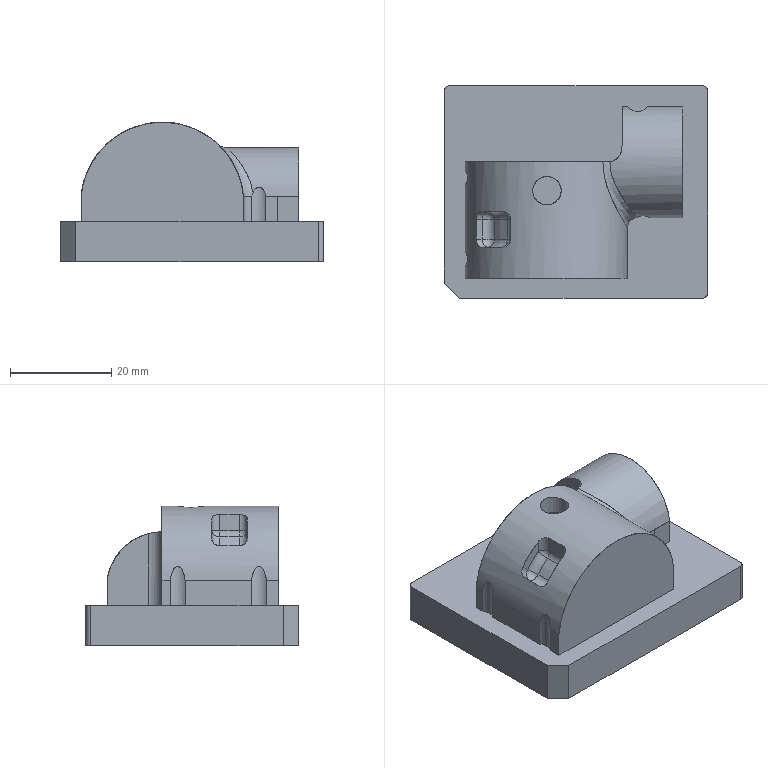NC program | PowerMill | posted with a generic post | part box 52 x 42 x 27.622 mm
Lines 1 to 940 of 322299:
%
O0001
N104 ( POWERMILL CB  : 2026004.0)
N105 ( POST VER      : 2026.0.0.5161)
N106 ( OPTION FILE   : FANUC)
N107 ( OUTPUT WORKPLANE : WORLD)
N108 (  )
N109 ( TOOL LIST )
N110 (---------------------------------------)
N111 ( NO. | ID        | DIA.| TIP RAD|LENGTH)
N112 (---------------------------------------)
N113 (    1|D10C_1_1_1 |10.0 |  0.0   |83.08 )
N114 (    2|D4C_1_1    | 4.0 |  0.0   | 74.8 )
N115 (   28|D2C_1_1    | 2.0 |  0.0   |67.72 )
N116 (    3|D10_1_1_1  |10.0 |  0.0   | 82.8 )
N117 (    7|R2_1_1     | 4.0 |  2.0   |71.76 )
N118 (   10|D3_1_1     | 3.0 |  0.0   |74.88 )
N119 (    4|R1_1_1     | 2.0 |  1.0   |64.72 )
N120 (   13|TEXT_D4_1_1| 4.0 |  0.3   |74.88 )
N121 (---------------------------------------)
N122 (  )
N123 ( NUMBER OF TOOLPATHS: 13.0 )
N124 ( ESTIMATED PROGRAM DURATION: 0 HOURS 30 MIN 34 SEC)
N125 (  )
N126 G00 G21 G80 G40 G17
N127 G90
N128 G54
N129 G53 Z0.0
N130 (---------------)
N131 ( START TOOLPATH : 精公开粗01-扫面平行-D10C )
N132 (---------------)
N133 ( TOOL NO.    :1 )
N134 ( TOOL TYPE   : ENDMILL)
N135 ( TOOL ID     : D10C_1_1_1)
N136 ( TOOL DIA    : 10.0 LENGTH 83.08)
N137 T1
N138 M6
N139 S8000 M03
N140 G00 G90 X0.0 Y0.0
N141 G43 Z10.2 H1
N142
N143 G05 P10000 R4
N144 X28.78 Y23.78
N145 Z1.132
N146 G01 Z-0.068 F6000.0
N147 X-28.78 F10000.0
N148 Y17.835
N149 X28.78
N150 Y11.89
N151 X-28.78
N152 Y5.945
N153 X28.78
N154 Y0.0
N155 X-28.78
N156 Y-5.945
N157 X28.78
N158 Y-11.89
N159 X-28.78
N160 Y-17.835
N161 X28.78
N162 Y-23.78
N163 X-28.78
N164 X-33.78
N165 G00 Z10.2
N166 G05 P0
N167 (---------------)
N168 ( END TOOLPATH : 精公开粗01-扫面平行-D10C )
N169 (---------------)
N170 ( START TOOLPATH : 精公开粗01-外形偏置-D10C )
N171 (---------------)
N172 G00 X-0.4155 Y-0.186 Z9.882
N173 G05 P10000 R4
N174 X2.3999 Y-30.215
N175 Z0.6838
N176 G01 Z-0.5162 F6000.0
N177 Y-29.6875 F10000.0
N178 G03 X-2.3476 Y-24.94 I-4.7475 J0.0
N179 G01 X-28.709
N180 G02 X-29.709 Y-23.94 I0.0 J1.0
N181 G01 Y23.568
N182 G02 X-28.709 Y24.568 I1.0 J0.0
N183 G01 X27.878
N184 G02 X28.878 Y23.568 I0.0 J-1.0
N185 G01 Y-0.2313
N186 X22.9872 Y-0.2546
N187 X17.4174 Y-0.2767
N188 X17.3721 Y11.1517
N189 G03 X15.2157 Y13.0657 I-1.9344 J-0.0077
N190 G03 X13.5525 Y10.7105 I0.222 J-1.9217
N191 G01 X14.089 Y8.3779
N192 G02 X14.5687 Y3.9884 I-18.4003 J-4.2319
N193 G01 X14.4374 Y-11.7373
N194 G03 X15.5858 Y-12.9585 I1.2128 J-0.0101
N195 G01 X16.1164 Y-12.9867
N196 G03 X17.4626 Y-11.705 I0.0678 J1.2766
N197 G01 X17.4174 Y-0.2767
N198 X22.9872 Y-0.2546
N199 Y-17.0492
N200 G02 X21.0004 Y-19.0491 I-2.0 J0.0
N201 G01 X10.7449 Y-19.1171
N202 G02 X8.7319 Y-17.0871 I-0.0133 J2.0
N203 G01 X9.0472 Y3.9049
N204 G03 X-5.0505 Y17.6259 I-13.5283 J0.2032
N205 G01 X-7.8978 Y17.506
N206 G03 X-21.0318 Y3.2025 I0.5776 J-13.7122
N207 G01 X-20.1558 Y-17.1107
N208 G02 X-21.6983 Y-18.9728 I-1.8015 J-0.0776
N209 G01 X-22.0663 Y-19.0263
N210 G02 X-24.1285 Y-17.2253 I-0.259 J1.7846
N211 G01 X-23.8181 Y16.6955
N212 G02 X-21.8182 Y18.6772 I1.9999 J-0.0183
N213 G01 X20.9872
N214 G02 X22.9872 Y16.6772 I0.0 J-2.0
N215 G01 Y-0.2546
N216 X28.878 Y-0.2313
N217 Y-23.94
N218 G02 X27.878 Y-24.94 I-1.0 J0.0
N219 G01 X-2.3476
N220 X-2.3491 Y-22.432
N221 X-9.3099 Y-22.4361
N222 X-10.0833 Y-22.3648
N223 X-10.8568 Y-22.1889
N224 X-11.6302 Y-21.889
N225 X-12.4036 Y-21.4357
N226 X-12.8677 Y-21.0685
N227 X-13.177 Y-20.7678
N228 X-13.5777 Y-20.2951
N229 X-14.06 Y-19.5217
N230 X-14.3759 Y-18.7482
N231 X-14.5593 Y-17.9748
N232 X-14.6224 Y-17.2014
N233 X-14.6405 Y-13.3343
N234 X-14.6103 Y-12.5608
N235 X-14.6019 Y-10.2405
N236 X-14.6459 Y-9.4671
N237 X-14.6072 Y-0.9594
N238 X-14.6415 Y1.3609
N239 X-14.6073 Y5.228
N240 X-14.6321 Y6.0014
N241 X-14.5643 Y6.7748
N242 X-14.3779 Y7.5483
N243 X-14.0567 Y8.3217
N244 X-13.576 Y9.0951
N245 X-13.177 Y9.5623
N246 X-12.8477 Y9.8685
N247 X-12.4036 Y10.223
N248 X-11.6892 Y10.642
N249 X-10.8568 Y10.9701
N250 X-10.0833 Y11.1451
N251 X-9.3099 Y11.2163
N252 X-2.3491 Y11.2116
N253 X-1.5756 Y11.1233
N254 X-0.8022 Y10.9323
N255 X-0.0807 Y10.642
N256 X0.7446 Y10.1386
N257 X1.0811 Y9.8685
N258 X1.5181 Y9.4317
N259 X1.7998 Y9.0951
N260 X2.2915 Y8.3058
N261 X2.6078 Y7.5483
N262 X2.7924 Y6.7748
N263 X2.8611 Y6.0014
N264 X2.8419 Y5.228
N265 X2.8774 Y0.5874
N266 X2.8333 Y-0.9594
N267 Y-0.9666
N268 Y-11.7874
N269 X2.8744 Y-13.3343
N270 X2.8668 Y-17.2014
N271 X2.8067 Y-17.9748
N272 X2.6234 Y-18.7482
N273 X2.303 Y-19.5217
N274 X1.826 Y-20.2951
N275 X1.5181 Y-20.6639
N276 X1.1107 Y-21.0685
N277 X0.7446 Y-21.3656
N278 X-0.0286 Y-21.8419
N279 X-0.8022 Y-22.1586
N280 X-1.5756 Y-22.348
N281 X-2.3491 Y-22.432
N282 X-2.3476 Y-24.94
N283 G00 Z3.2856
N284 G01 X2.3999 Y-30.215
N285 G00 Z0.2856
N286 G01 Z-0.9144 F6000.0
N287 Y-29.6875 F10000.0
N288 G03 X-2.3476 Y-24.94 I-4.7475 J0.0
N289 G01 X-28.709
N290 G02 X-29.709 Y-23.94 I0.0 J1.0
N291 G01 Y23.568
N292 G02 X-28.709 Y24.568 I1.0 J0.0
N293 G01 X27.878
N294 G02 X28.878 Y23.568 I0.0 J-1.0
N295 G01 Y-0.2845
N296 X22.9872 Y-0.2788
N297 X17.0576 Y-0.273
N298 X17.0697 Y12.19
N299 G03 X16.5006 Y12.7597 I-0.5692 J0.0005
N300 G01 X15.1565 Y12.7598
N301 G03 X14.8346 Y12.2613 I-0.0001 J-0.3531
N302 G01 X15.0028 Y11.889
N303 G02 X16.6841 Y3.5678 I-17.346 J-7.8354
N304 G01 X16.2681 Y-12.7268
N305 G03 X16.5196 Y-13.0878 I0.3713 J-0.0095
N306 G01 X16.5426 Y-13.0956
N307 G03 X17.0455 Y-12.736 I0.1226 J0.3599
N308 G01 X17.0576 Y-0.273
N309 X22.9872 Y-0.2788
N310 Y-17.0492
N311 G02 X21.0033 Y-19.0491 I-2.0 J0.0
N312 G01 X12.2098 Y-19.1201
N313 G02 X10.1945 Y-17.0647 I-0.0161 J1.9999
N314 G01 X10.7699 Y3.6831
N315 G03 X-1.6795 Y17.1746 I-13.1402 J0.3644
N316 G01 X-8.0692 Y17.5108
N317 G03 X-22.4796 Y3.2616 I-0.7199 J-13.6832
N318 G01 X-21.6108 Y-17.7521
N319 G02 X-22.5168 Y-18.7408 I-0.9496 J-0.0393
N320 G01 X-23.1117 Y-18.7681
N321 G02 X-24.1057 Y-17.8108 I-0.0436 J0.9494
N322 G01 X-23.8181 Y16.6938
N323 G02 X-21.8182 Y18.6772 I1.9999 J-0.0166
N324 G01 X20.9872
N325 G02 X22.9872 Y16.6772 I0.0 J-2.0
N326 G01 Y-0.2788
N327 X28.878 Y-0.2845
N328 Y-23.94
N329 G02 X27.878 Y-24.94 I-1.0 J0.0
N330 G01 X-0.7722
N331 X-0.8022 Y-22.432
N332 X-1.5756 Y-22.4412
N333 X-10.0833
N334 X-10.8568 Y-22.4363
N335 X-11.6302 Y-22.3544
N336 X-12.4036 Y-22.1649
N337 X-13.1939 Y-21.8419
N338 X-13.9505 Y-21.3731
N339 X-14.3262 Y-21.0685
N340 X-14.7239 Y-20.6762
N341 X-15.0415 Y-20.2951
N342 X-15.4973 Y-19.5621
N343 X-15.8358 Y-18.7482
N344 X-16.0184 Y-17.9748
N345 X-16.0829 Y-17.2014
N346 X-16.0644 Y-14.1077
N347 X-16.0897 Y-13.3343
N348 X-16.0907 Y6.0014
N349 X-16.0284 Y6.7748
N350 X-15.8421 Y7.5483
N351 X-15.5215 Y8.3217
N352 X-15.0371 Y9.0951
N353 X-14.7239 Y9.4705
N354 X-14.3198 Y9.8685
N355 X-13.9505 Y10.1626
N356 X-13.177 Y10.6358
N357 X-12.4036 Y10.9477
N358 X-11.6302 Y11.1341
N359 X-10.8568 Y11.2158
N360 X-10.0833 Y11.2213
N361 X-1.5756
N362 X-0.8022 Y11.2116
N363 X-0.0288 Y11.1164
N364 X0.7446 Y10.9135
N365 X1.3993 Y10.642
N366 X2.2915 Y10.083
N367 X2.5549 Y9.8685
N368 X3.0649 Y9.3467
N369 X3.27 Y9.0951
N370 X3.7539 Y8.3217
N371 X4.0784 Y7.5483
N372 X4.2652 Y6.7748
N373 X4.3314 Y6.0014
N374 X4.3208 Y5.228
N375 X4.3392 Y2.9077
N376 X4.3034 Y-1.7329
N377 X4.306 Y-12.5608
N378 X4.3287 Y-13.3343
N379 X4.3095 Y-14.1077
N380 Y-14.1154
N381 X4.3286 Y-17.2014
N382 X4.2638 Y-17.9748
N383 X4.0806 Y-18.7482
N384 X3.7637 Y-19.5217
N385 X3.2835 Y-20.2951
N386 X3.0649 Y-20.5654
N387 X2.5735 Y-21.0685
N388 X2.2915 Y-21.3024
N389 X1.4359 Y-21.8419
N390 X0.7446 Y-22.1331
N391 X-0.0288 Y-22.3371
N392 X-0.8022 Y-22.432
N393 X-0.7722 Y-24.94
N394 X-2.3476
N395 G00 Z2.8874
N396 G01 X2.3999 Y-30.215
N397 G00 Z-0.1126
N398 G01 Z-1.3126 F6000.0
N399 Y-29.6875 F10000.0
N400 G03 X-2.3476 Y-24.94 I-4.7475 J0.0
N401 G01 X-28.709
N402 G02 X-29.709 Y-23.94 I0.0 J1.0
N403 G01 Y23.568
N404 G02 X-28.709 Y24.568 I1.0 J0.0
N405 G01 X27.878
N406 G02 X28.878 Y23.568 I0.0 J-1.0
N407 G01 Y-0.518
N408 X23.0842 Y-0.5088
N409 X17.7571 Y-0.5003
N410 X17.7771 Y12.1344
N411 G03 X16.4479 Y13.4671 I-1.3306 J0.0021
N412 G01 X16.1198 Y13.4675
N413 G03 X15.3545 Y12.3375 I-0.0009 J-0.8236
N414 G01 X15.6519 Y11.5956
N415 G02 X16.8882 Y4.9198 I-16.0082 J-6.4169
N416 G01 X16.6172 Y-13.1236
N417 G03 X17.0637 Y-13.5815 I0.4511 J-0.0068
N418 G01 X17.283 Y-13.5838
N419 G03 X17.737 Y-13.135 I0.0045 J0.4495
N420 G01 X17.7571 Y-0.5003
N421 X23.0842 Y-0.5088
N422 Y-17.7235
N423 G02 X21.6615 Y-19.1462 I-1.4227 J0.0
N424 G01 X12.4578 Y-19.1463
N425 G02 X11.1881 Y-17.7948 I0.0 J1.2722
N426 G01 X11.1976 Y-17.6086
N427 X11.5863 Y4.9572
N428 G03 X-0.2272 Y17.169 I-12.0047 J0.2068
N429 G01 X-10.8025 Y17.3375
N430 G03 X-23.3444 Y4.7809 I-0.1966 J-12.3455
N431 G01 X-22.9698 Y-17.1238
N432 X-22.8718 Y-18.4412
N433 G02 X-23.2256 Y-18.837 I-0.3667 J-0.0283
N434 G01 X-23.5239 Y-18.8474
N435 G02 X-23.9045 Y-18.48 I-0.0128 J0.3675
N436 G01 X-23.9152 Y17.3511
N437 G02 X-22.4925 Y18.7742 I1.4227 J0.0004
N438 G01 X21.6615
N439 G02 X23.0842 Y17.3515 I0.0 J-1.4227
N440 G01 Y-0.5088
N441 X28.878 Y-0.518
N442 Y-23.94
N443 G02 X27.878 Y-24.94 I-1.0 J0.0
N444 G01 X0.418
N445 X0.2612 Y-22.4231
N446 X-0.0288 Y-22.4412
N447 X-11.6302
N448 X-12.4036 Y-22.4056
N449 X-13.177 Y-22.2655
N450 X-13.9505 Y-22.003
N451 X-14.297 Y-21.8419
N452 X-14.7239 Y-21.601
N453 X-15.4287 Y-21.0685
N454 X-16.137 Y-20.2951
N455 X-16.2707 Y-20.1076
N456 X-16.6157 Y-19.5217
N457 X-16.934 Y-18.7482
N458 X-17.1168 Y-17.9748
N459 X-17.1785 Y-17.2014
N460 X-17.1744 Y-14.1077
N461 X-17.1585 Y-12.5608
N462 X-17.1779 Y-9.4671
N463 X-17.1614 Y-0.186
N464 X-17.1782 Y0.5874
N465 X-17.1707 Y6.0014
N466 X-17.1024 Y6.7748
N467 X-16.9162 Y7.5483
N468 X-16.5963 Y8.3217
N469 X-16.2707 Y8.8703
N470 X-16.1117 Y9.0951
N471 X-15.4973 Y9.7733
N472 X-14.7239 Y10.3707
N473 X-14.2483 Y10.642
N474 X-13.9505 Y10.7779
N475 X-13.177 Y11.0406
N476 X-12.4036 Y11.1831
N477 X-11.6302 Y11.2213
N478 X-0.0288 Y11.2214
N479 X0.7446 Y11.1717
N480 X1.5181 Y11.0156
N481 X2.4979 Y10.642
N482 X3.0649 Y10.3117
N483 X3.6435 Y9.8685
N484 X3.8383 Y9.686
N485 X4.3612 Y9.0951
N486 X4.6118 Y8.7226
N487 X4.8439 Y8.3217
N488 X5.1639 Y7.5483
N489 X5.3525 Y6.7748
N490 X5.4166 Y6.0014
N491 X5.4212 Y2.9077
N492 X5.3948 Y-0.9594
N493 Y-12.5608
N494 X5.3952 Y-12.5702
N495 X5.4238 Y-13.3343
N496 X5.4247 Y-17.2014
N497 X5.3624 Y-17.9748
N498 X5.1795 Y-18.7482
N499 X4.8619 Y-19.5217
N500 X4.6118 Y-19.9596
N501 X4.3822 Y-20.2951
N502 X3.8383 Y-20.9144
N503 X3.6741 Y-21.0685
N504 X3.0649 Y-21.5384
N505 X2.5426 Y-21.8419
N506 X2.2915 Y-21.9626
N507 X1.5181 Y-22.2387
N508 X0.7446 Y-22.393
N509 X0.2612 Y-22.4231
N510 X0.418 Y-24.94
N511 X-2.3476
N512 G00 Z2.4892
N513 G01 X2.3999 Y-30.215
N514 G00 Z-0.5108
N515 G01 Z-1.7108 F6000.0
N516 Y-29.6875 F10000.0
N517 G03 X-2.3476 Y-24.94 I-4.7475 J0.0
N518 G01 X-28.709
N519 G02 X-29.709 Y-23.94 I0.0 J1.0
N520 G01 Y23.568
N521 G02 X-28.709 Y24.568 I1.0 J0.0
N522 G01 X27.878
N523 G02 X28.878 Y23.568 I0.0 J-1.0
N524 G01 Y-0.1777
N525 X23.1783 Y-0.1895
N526 X18.5438 Y-0.199
N527 X18.5172 Y12.6516
N528 G03 X16.6909 Y14.2143 I-1.5844 J-0.0032
N529 G03 X15.4212 Y12.1734 I0.2419 J-1.5659
N530 G01 X15.9354 Y10.5368
N531 G02 X16.6565 Y5.8812 I-14.9633 J-4.7014
N532 G01 X16.7119 Y-13.0537
N533 G03 X17.5048 Y-13.8443 I0.7929 J0.0023
N534 G01 X17.7773
N535 G03 X18.5703 Y-13.0497 I0.0 J0.7929
N536 G01 X18.5438 Y-0.199
N537 X23.1783 Y-0.1895
N538 Y-18.8932
N539 G02 X22.8312 Y-19.2403 I-0.3471 J0.0
N540 G01 X12.1493 Y-19.2404
N541 G02 X11.8751 Y-18.9269 I0.0 J0.2767
N542 G01 X11.929 Y-18.5253
N543 G03 X12.112 Y-15.7107 I-20.433 J2.7418
N544 G01 X12.1006 Y-12.4824
N545 X12.0566 Y5.8315
N546 G03 X0.7861 Y17.0039 I-11.1995 J-0.0269
N547 G01 X-12.3889 Y16.9203
N548 X-13.0327 Y16.9096
N549 X-13.5164 Y16.8882
N550 X-13.9983 Y16.8402
N551 X-14.1741 Y16.8179
N552 G03 X-16.2787 Y16.3267 I1.3322 J-10.4639
N553 G01 X-16.4753 Y16.259
N554 X-16.9889 Y16.0651
N555 X-17.4903 Y15.8416
N556 X-17.6232 Y15.7777
N557 X-17.9323 Y15.6215
N558 X-18.2352 Y15.4536
N559 X-18.314 Y15.4079
N560 G03 X-21.1188 Y13.0623 I5.3868 J-9.2909
N561 G01 X-21.2302 Y12.9309
N562 G03 X-22.4592 Y11.1191 I7.802 J-6.615
N563 G01 X-22.495 Y11.0517
N564 X-22.7031 Y10.6365
N565 X-22.8908 Y10.2117
N566 X-22.9648 Y10.0326
N567 G03 X-23.4415 Y8.5639 I9.1626 J-3.7856
N568 G01 X-23.4708 Y8.4419
N569 G03 X-23.7434 Y6.5319 I9.9814 J-2.3991
N570 G01 X-23.7604 Y6.1656
N571 X-23.7859 Y-7.0983
N572 X-23.7679 Y-17.3085
N573 X-23.7652 Y-17.4079
N574 X-23.6871 Y-18.4372
N575 X-23.6293 Y-19.0061
N576 X-23.6475 Y-19.0997
N577 X-23.7148 Y-19.1672
N578 X-23.7447 Y-19.1832
N579 G02 X-24.0076 Y-19.0257 I-0.0842 J0.1575
N580 G01 X-24.0093 Y18.5212
N581 G02 X-23.6622 Y18.8683 I0.3471 J0.0
N582 G01 X22.8312
N583 G02 X23.1783 Y18.5212 I0.0 J-0.3471
N584 G01 Y-0.1895
N585 X28.878 Y-0.1777
N586 Y-23.94
N587 G02 X27.878 Y-24.94 I-1.0 J0.0
N588 G01 X0.945
N589 X0.8413 Y-22.4372
N590 X0.7446 Y-22.4412
N591 X-12.4036
N592 X-13.177 Y-22.4173
N593 X-13.9505 Y-22.2955
N594 X-14.7239 Y-22.0533
N595 X-15.1937 Y-21.8419
N596 X-15.4973 Y-21.6728
N597 X-16.2707 Y-21.1106
N598 X-17.0293 Y-20.2951
N599 X-17.5083 Y-19.5217
N600 X-17.8243 Y-18.7482
N601 X-18.0071 Y-17.9748
N602 X-18.0705 Y-17.2014
N603 X-18.0513 Y-11.014
N604 X-18.0793 Y-9.4671
N605 X-18.0796 Y-4.8266
N606 X-18.0566 Y-2.5063
N607 X-18.064 Y6.0014
N608 X-17.9972 Y6.7748
N609 X-17.8113 Y7.5483
N610 X-17.4918 Y8.3217
N611 X-17.0442 Y9.0447
N612 X-16.2941 Y9.8685
N613 X-15.4973 Y10.4502
N614 X-15.1511 Y10.642
N615 X-14.7239 Y10.8331
N616 X-13.9505 Y11.0751
N617 X-13.177 Y11.1983
N618 X-12.4036 Y11.2214
N619 X0.7446
N620 X1.5181 Y11.1904
N621 X2.2915 Y11.0547
N622 X3.0649 Y10.797
N623 X3.4073 Y10.642
N624 X3.8383 Y10.3985
N625 X4.5503 Y9.8685
N626 X5.2645 Y9.0951
N627 X5.7482 Y8.3217
N628 X6.0676 Y7.5483
N629 X6.2533 Y6.7748
N630 X6.3197 Y6.0014
N631 X6.2994 Y5.228
N632 X6.317 Y0.5874
N633 X6.2997 Y-0.9594
N634 X6.2994 Y-12.5608
N635 X6.2995 Y-12.5667
N636 X6.3174 Y-13.3343
N637 X6.315 Y-17.2014
N638 X6.2515 Y-17.9748
N639 X6.0687 Y-18.7482
N640 X5.7527 Y-19.5217
N641 X5.2738 Y-20.2951
N642 X4.6118 Y-21.0251
N643 X3.8383 Y-21.6139
N644 X3.4382 Y-21.8419
N645 X3.0649 Y-22.0143
N646 X2.2915 Y-22.2706
N647 X1.5181 Y-22.4092
N648 X0.8413 Y-22.4372
N649 X0.945 Y-24.94
N650 X-2.3476
N651 G00 Z2.091
N652 G01 X2.3999 Y-30.215
N653 G00 Z-0.909
N654 G01 Z-2.109 F6000.0
N655 Y-29.6875 F10000.0
N656 G03 X-2.3476 Y-24.94 I-4.7475 J0.0
N657 G01 X-5.8295
N658 Y-22.4412
N659 X-13.177
N660 X-13.9505 Y-22.4204
N661 X-14.7239 Y-22.2964
N662 X-15.4973 Y-22.0556
N663 X-15.9697 Y-21.8419
N664 X-16.2707 Y-21.6738
N665 X-17.0442 Y-21.1102
N666 X-17.8002 Y-20.2951
N667 X-18.2781 Y-19.5217
N668 X-18.5945 Y-18.7482
N669 X-18.777 Y-17.9748
N670 X-18.8402 Y-17.2014
N671 X-18.845 Y-13.3343
N672 X-18.8431 Y-10.2405
N673 X-18.7258 Y-9.4671
N674 X-18.4835 Y-8.6937
N675 X-18.2375 Y-8.1716
N676 X-18.2019 Y-8.0678
N677 X-18.1898 Y-7.9587
N678 X-18.1893 Y-6.8746
N679 X-18.2031 Y-6.758
N680 X-18.2436 Y-6.6479
N681 X-18.383 Y-6.3734
N682 X-18.6659 Y-5.6
N683 X-18.8196 Y-4.8266
N684 X-18.8589 Y-4.0531
N685 X-18.8425 Y-0.186
N686 X-18.8496 Y6.0014
N687 X-18.7832 Y6.7748
N688 X-18.591 Y7.5637
N689 X-18.2783 Y8.3217
N690 X-17.7955 Y9.0951
N691 X-17.0826 Y9.8685
N692 X-16.2707 Y10.4606
N693 X-15.9427 Y10.642
N694 X-15.4973 Y10.8411
N695 X-14.7239 Y11.081
N696 X-13.9505 Y11.2002
N697 X-13.177 Y11.2214
N698 X-5.767 Y11.2213
N699 X0.7446
N700 X0.7457
N701 X1.5181
N702 X2.2915 Y11.1927
N703 X3.0649 Y11.058
N704 X3.8383 Y10.8015
N705 X4.1898 Y10.642
N706 X4.6118 Y10.4043
N707 X5.3295 Y9.8685
N708 X6.0443 Y9.0951
N709 X6.5273 Y8.3217
N710 X6.8466 Y7.5483
N711 X7.0324 Y6.7748
N712 X7.0988 Y6.0014
N713 X7.0864 Y5.228
N714 X7.1006 Y-0.186
N715 X7.1011 Y-13.3343
N716 X7.0752 Y-14.1077
N717 X7.0849 Y-17.2014
N718 X7.0212 Y-17.9748
N719 X6.8386 Y-18.7482
N720 X6.5232 Y-19.5217
N721 X6.0447 Y-20.2951
N722 X5.3852 Y-21.0257
N723 X4.6118 Y-21.6148
N724 X4.214 Y-21.8419
N725 X3.8383 Y-22.0164
N726 X3.0649 Y-22.2735
N727 X2.2915 Y-22.411
N728 X1.5181 Y-22.4412
N729 X-5.8295
N730 Y-24.94
N731 X-28.709
N732 G02 X-29.709 Y-23.94 I0.0 J1.0
N733 G01 Y23.568
N734 G02 X-28.709 Y24.568 I1.0 J0.0
N735 G01 X27.878
N736 G02 X28.878 Y23.568 I0.0 J-1.0
N737 G01 Y-0.3507
N738 X23.7641 Y-0.3509
N739 X18.3806 Y-0.351
N740 X18.3802 Y13.2692
N741 G03 X17.5793 Y14.0702 I-0.801 J0.0
N742 G01 X16.2076 Y14.0705
N743 G03 X15.7894 Y13.388 I-0.0001 J-0.4693
N744 G01 X16.0177 Y12.9402
N745 G02 X17.7694 Y5.7072 I-14.3041 J-7.2927
N746 G01 X17.8403 Y-13.9721
N747 G03 X18.077 Y-14.208 I0.2367 J0.0008
N748 G01 X18.1443
N749 G03 X18.3811 Y-13.9713 I0.0 J0.2367
N750 G01 X18.3806 Y-0.351
N751 X23.7641 Y-0.3509
N752 Y-18.8872
N753 G02 X22.8252 Y-19.8261 I-0.9389 J0.0
N754 G01 X12.7541 Y-19.8262
N755 G02 X12.0469 Y-19.0207 I0.0 J0.7132
N756 G01 X12.1765 Y-18.0272
N757 G03 X12.4652 Y-13.4436 I-34.0753 J4.4464
N758 G01 X12.3888 Y5.6813
N759 G03 X1.6856 Y16.3461 I-10.7075 J-0.0428
N760 G01 X-13.3987 Y16.3521
N761 G03 X-24.1682 Y5.6513 I-0.0043 J-10.7654
N762 G01 X-24.2071 Y-0.8435
N763 G03 X-24.0596 Y-4.0664 I31.1978 J-0.1871
N764 G01 X-23.7513 Y-7.2202
N765 X-23.7418 Y-7.4205
N766 X-23.7524 Y-7.6207
N767 X-24.0636 Y-10.628
N768 G03 X-24.1437 Y-14.2707 I22.3625 J-2.3141
N769 G01 X-23.9167 Y-18.0497
N770 X-23.7787 Y-19.29
N771 G02 X-23.9895 Y-19.6263 I-0.3163 J-0.036
N772 G01 X-24.1102 Y-19.6688
N773 G02 X-24.5886 Y-19.3298 I-0.1191 J0.339
N774 G01 X-24.5951 Y18.5151
N775 G02 X-23.6562 Y19.4541 I0.9389 J0.0001
N776 G01 X22.8252
N777 G02 X23.7641 Y18.5152 I0.0 J-0.9389
N778 G01 Y-0.3509
N779 X28.878 Y-0.3507
N780 Y-23.94
N781 G02 X27.878 Y-24.94 I-1.0 J0.0
N782 G01 X-2.3476
N783 G00 Z1.6928
N784 G01 X2.3999 Y-30.215
N785 G00 Z-1.3072
N786 G01 Z-2.5072 F6000.0
N787 Y-29.6875 F10000.0
N788 G03 X-2.3476 Y-24.94 I-4.7475 J0.0
N789 G01 X-28.709
N790 G02 X-29.709 Y-23.94 I0.0 J1.0
N791 G01 Y23.568
N792 G02 X-28.709 Y24.568 I1.0 J0.0
N793 G01 X27.878
N794 G02 X28.878 Y23.568 I0.0 J-1.0
N795 G01 Y-0.2917
N796 X23.942
N797 X18.5033
N798 X18.5034 Y13.7698
N799 G03 X18.0798 Y14.1934 I-0.4236 J0.0
N800 G01 X16.2408 Y14.1935
N801 G03 X16.0281 Y13.8295 I0.0 J-0.2441
N802 G01 X16.1776 Y13.5642
N803 G02 X18.2209 Y5.7343 I-13.8148 J-7.7866
N804 G01 X18.166 Y-14.3526
N805 G03 X18.2908 Y-14.478 I0.125 J-0.0004
N806 G01 X18.378 Y-14.4781
N807 G03 X18.5032 Y-14.3531 I0.0002 J0.125
N808 G01 X18.5033 Y-0.2917
N809 X23.942
N810 Y-19.5626
N811 G02 X23.5006 Y-20.004 I-0.4414 J0.0
N812 G01 X12.7479
N813 G02 X12.4179 Y-19.5769 I0.0 J0.341
N814 G01 X12.4535 Y-19.4405
N815 G03 X12.67 Y-18.1174 I-6.9802 J1.8214
N816 G01 X12.7187 Y-17.3973
N817 X12.784 Y5.7442
N818 G03 X2.3393 Y16.2102 I-10.437 J0.0289
N819 G01 X-14.1825 Y16.1981
N820 G03 X-24.4806 Y6.0264 I0.0075 J-10.3065
N821 G01 X-24.5904 Y-2.3671
N822 G03 X-24.1213 Y-6.6813 I17.9199 J-0.2343
N823 G01 X-24.0438 Y-7.0131
N824 G02 X-24.0625 Y-7.9974 I-1.9475 J-0.4553
N825 G01 X-24.1102 Y-8.1713
N826 X-24.1744 Y-8.4171
N827 X-24.2325 Y-8.6643
N828 X-24.2543 Y-8.7623
N829 G03 X-24.5082 Y-11.1266 I10.4135 J-2.3142
N830 G01 X-24.4785 Y-17.2947
N831 X-24.4367 Y-17.9922
N832 X-24.3783 Y-18.5828
N833 X-24.2757 Y-19.1673
N834 X-24.1776 Y-19.6243
N835 G02 X-24.4405 Y-19.9874 I-0.2947 J-0.0633
N836 G02 X-24.7738 Y-19.6876 I-0.0318 J0.2998
N837 G01 X-24.773 Y19.1906
N838 G02 X-24.3316 Y19.632 I0.4414 J0.0
N839 G01 X23.5006
N840 G02 X23.942 Y19.1906 I0.0 J-0.4414
N841 G01 Y-0.2917
N842 X28.878
N843 Y-23.94
N844 G02 X27.878 Y-24.94 I-1.0 J0.0
N845 G01 X2.6045
N846 X2.4848 Y-22.432
N847 X2.2915 Y-22.4412
N848 X-13.9505
N849 X-14.7239 Y-22.4146
N850 X-15.4973 Y-22.2827
N851 X-16.2707 Y-22.029
N852 X-16.6788 Y-21.8419
N853 X-17.0442 Y-21.6335
N854 X-17.8001 Y-21.0685
N855 X-18.5037 Y-20.2951
N856 X-18.9839 Y-19.5217
N857 X-19.2974 Y-18.7482
N858 X-19.48 Y-17.9748
N859 X-19.5444 Y-17.2014
N860 X-19.5432 Y-11.014
N861 X-19.5027 Y-10.2405
N862 X-19.3644 Y-9.5426
N863 X-19.0582 Y-8.6937
N864 X-18.591 Y-7.8846
N865 X-18.4678 Y-7.7278
N866 G03 X-18.4414 Y-7.1468 I-0.3932 J0.3089
N867 G01 X-18.9412 Y-6.3734
N868 X-19.2733 Y-5.6
N869 X-19.465 Y-4.8266
N870 X-19.5436 Y-4.0531
N871 X-19.5368 Y6.0014
N872 X-19.4705 Y6.7748
N873 X-19.2848 Y7.5483
N874 X-18.9656 Y8.3217
N875 X-18.4828 Y9.0951
N876 X-17.8176 Y9.8246
N877 X-17.0442 Y10.4087
N878 X-16.6298 Y10.642
N879 X-16.2707 Y10.8054
N880 X-15.4973 Y11.0606
N881 X-14.7239 Y11.1931
N882 X-13.9505 Y11.2214
N883 X2.2915
N884 X3.0649 Y11.1843
N885 X3.8383 Y11.037
N886 X4.6118 Y10.7687
N887 X4.8808 Y10.642
N888 X5.3852 Y10.3524
N889 X6.1586 Y9.7419
N890 X6.7342 Y9.0951
N891 X6.9321 Y8.8135
N892 X7.2177 Y8.3217
N893 X7.5356 Y7.5483
N894 X7.7055 Y6.8659
N895 X7.7875 Y6.0014
N896 X7.7901 Y2.9077
N897 X7.7668 Y-0.9594
N898 Y-12.5608
N899 X7.7898 Y-13.3343
N900 X7.7878 Y-17.2014
N901 X7.7244 Y-17.9748
N902 X7.542 Y-18.7482
N903 X7.2271 Y-19.5217
N904 X6.9321 Y-20.0338
N905 X6.7486 Y-20.2951
N906 X6.1586 Y-20.9624
N907 X5.3852 Y-21.5726
N908 X4.922 Y-21.8419
N909 X4.6118 Y-21.9894
N910 X3.8383 Y-22.2581
N911 X3.0649 Y-22.4043
N912 X2.4848 Y-22.432
N913 X2.6045 Y-24.94
N914 X-2.3476
N915 G00 Z1.2946
N916 G01 X2.3999 Y-30.215
N917 G00 Z-1.7054
N918 G01 Z-2.9054 F6000.0
N919 Y-29.6875 F10000.0
N920 G03 X-2.3476 Y-24.94 I-4.7475 J0.0
N921 G01 X-5.8295
N922 Y-22.4412
N923 X-14.7239
N924 X-15.4973 Y-22.3973
N925 X-16.2707 Y-22.2419
N926 X-17.0442 Y-21.9624
N927 X-17.296 Y-21.8419
N928 X-17.8176 Y-21.5327
N929 X-18.4175 Y-21.0685
N930 X-18.591 Y-20.9031
N931 X-19.1226 Y-20.2951
N932 X-19.3644 Y-19.9376
N933 X-19.5993 Y-19.5217
N934 X-19.9155 Y-18.7482
N935 X-20.0979 Y-17.9748
N936 X-20.1613 Y-17.2014
N937 X-20.1386 Y-16.428
N938 X-20.1501 Y-11.014
N939 X-20.1061 Y-10.2405
N940 X-19.9444 Y-9.4671
N941 X-19.7264 Y-8.8882
N942 X-24.5203 Y-7.49
N943 G02 X-24.7104 Y-7.4628 I-0.0931 J0.0272
N944 G01 Y-7.3518
N945 G02 X-24.5164 I0.097 J0.0
N946 G01 Y-7.4628
N947 X-24.5174 Y-7.4765
N948 X-24.5203 Y-7.49
N949 X-19.7264 Y-8.8882
N950 X-19.6531 Y-8.6937
N951 X-19.3644 Y-8.1633
N952 X-19.2053 Y-7.9203
N953 X-19.052 Y-7.7263
N954 G03 X-19.0382 Y-7.1243 I-0.3922 J0.3101
N955 G01 X-19.3644 Y-6.6705
N956 X-19.5371 Y-6.3734
N957 X-19.8713 Y-5.6
N958 X-20.0703 Y-4.8266
N959 X-20.1379 Y-4.2648
N960 X-20.1463 Y6.0014
N961 X-20.0797 Y6.7748
N962 X-19.8942 Y7.5483
N963 X-19.5754 Y8.3217
N964 X-19.3644 Y8.693
N965 X-19.0932 Y9.0951
N966 X-18.591 Y9.67
N967 X-18.3814 Y9.8685
N968 X-17.8176 Y10.3043
N969 X-17.0442 Y10.7374
N970 X-16.2707 Y11.0196
N971 X-15.4973 Y11.1768
N972 X-14.7239 Y11.2213
N973 X-13.9515
N974 X-13.9505
N975 X2.2915
N976 X2.2924
N977 X3.0649
N978 X3.8383 Y11.1653
N979 X4.6118 Y10.995
N980 X5.3852 Y10.6994
N981 X6.1586 Y10.2485
N982 X6.6404 Y9.8685
N983 X6.9321 Y9.5872
N984 X7.3512 Y9.0951
N985 X7.7055 Y8.5588
N986 X7.8347 Y8.3217
N987 X8.1531 Y7.5483
N988 X8.3379 Y6.7748
N989 X8.4045 Y6.0014
N990 X8.3869 Y5.228
N991 X8.3944 Y-0.186
N992 X8.3942 Y-11.7874
N993 X8.3831 Y-16.428
N994 X8.4057 Y-17.2014
N995 X8.3424 Y-17.9748
N996 X8.1599 Y-18.7482
N997 X7.8443 Y-19.5217
N998 X7.7055 Y-19.7771
N999 X7.367 Y-20.2951
N1000 X6.9321 Y-20.8057
N1001 X6.662 Y-21.0685
N1002 X6.1586 Y-21.4682
N1003 X5.5384 Y-21.8419
N1004 X4.6118 Y-22.2142
N1005 X3.8383 Y-22.3843
N1006 X3.0649 Y-22.4412
N1007 X-5.8295
N1008 Y-24.94
N1009 X-28.709
N1010 G02 X-29.709 Y-23.94 I0.0 J1.0
N1011 G01 Y23.568
N1012 G02 X-28.709 Y24.568 I1.0 J0.0
N1013 G01 X27.878
N1014 G02 X28.878 Y23.568 I0.0 J-1.0
N1015 G01 Y-0.4707
N1016 X24.0666 Y-0.4641
N1017 X19.1927 Y-0.4575
N1018 X19.2124 Y13.8956
N1019 G03 X18.2071 Y14.9024 I-1.0055 J0.0013
N1020 G01 X15.8874 Y14.9027
N1021 G03 X15.436 Y14.0722 I-0.0001 J-0.5378
N1022 G01 X15.7562 Y13.5785
N1023 G02 X18.5359 Y4.1943 I-14.4845 J-9.3944
N1024 G01 X18.5434 Y-8.4708
N1025 X18.5263 Y-10.053
N1026 X18.473 Y-11.6345
N1027 X18.3303 Y-14.7992
N1028 G03 X18.613 Y-15.1522 I0.3424 J-0.0155
N1029 G01 X18.7386 Y-15.1744
N1030 G03 X19.173 Y-14.8105 I0.0644 J0.3644
N1031 G01 X19.1927 Y-0.4575
N1032 X24.0666 Y-0.4641
N1033 Y-18.1286
N1034 G02 X22.1143 Y-20.128 I-2.0 J0.0
N1035 G01 X15.1375 Y-20.2945
N1036 G02 X13.0974 Y-18.1208 I-0.0477 J1.9995
N1037 G01 X13.4468 Y-14.1245